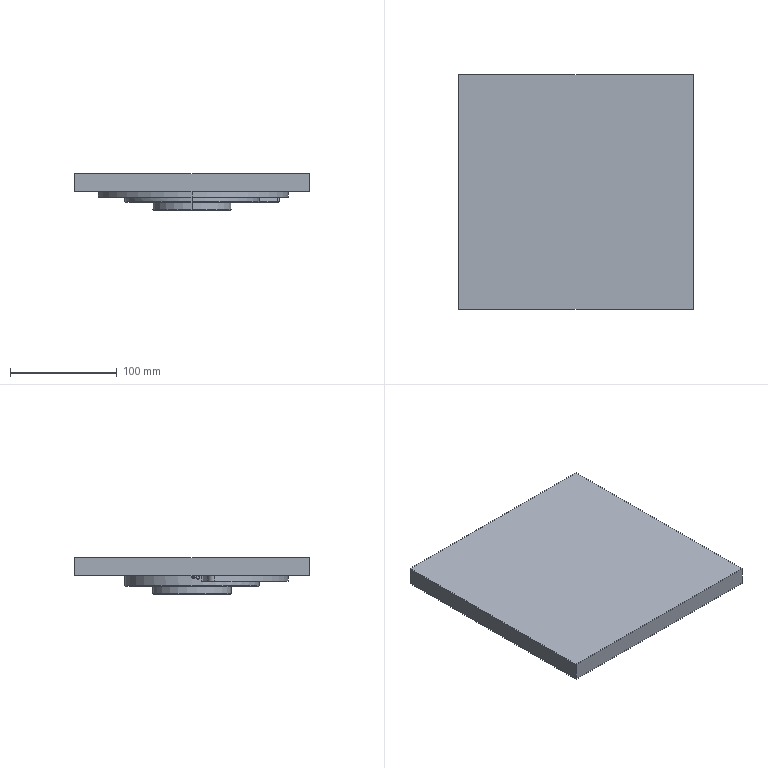NC program | NX | posted with a generic post | part box 220 x 220 x 34.5 mm
Lines 5366 to 5610 of 5610:
(FLOOR_WALL_COPY_COPY , TOOL : D10JING)
N10724 T07 M6
N10726 G54
N10728 G17 G0 G90 X-94.136 Y20.831 S9500 M3
N10730 G43 Z30. H7
N10732 Z-11.
N10734 G94 G1 Z-12.5 F1000.
N10736 X-93.972 Y20.821
N10738 G3 X-92.424 Y21.971 R1.5
N10740 G2 X87.34 Y-37.372 R-95.
N10742 G3 X82.185 Y-28.911 R8.5
N10744 G1 X65. Y-21.616
N10746 G3 X-68.148 Y6.939 R-68.5
N10748 G1 X-84.432 Y9.81
N10750 G2 X-92.424 Y21.971 R10.
N10752 G1 X-86.587 Y20.584
N10754 G2 X85.715 Y-23.956 R-89.
N10756 G3 X84.53 Y-23.388 R14.5
N10758 G1 X72.249 Y-18.175
N10760 G3 X-73.188 Y13.92 R-74.5
N10762 G1 X-83.39 Y15.719
N10764 G2 X-86.587 Y20.584 R4.
N10766 G1 X-80.232 Y21.255
N10768 G2 X81.522 Y-15.593 R83.
N10770 G1 X79.166 Y-14.593
N10772 G3 X-77.761 Y20.819 R80.5
N10774 G1 X-80.232 Y21.255
N10776 G3 X-81.902 Y20.291 R1.5
N10778 G1 Z-11.
N10780 G0 Z30.
N10782 X-69.419 Y3.355
N10784 Z-11.
N10786 G1 Z-12.5
N10788 X-69.173 Y3.38
N10790 G3 X-67.833 Y4.767 R1.5
N10792 G2 X64.379 Y-21.895 R-68.
N10794 G1 X81.99 Y-29.371
N10796 G2 X86.282 Y-39.729 R8.
N10798 G3 X86.879 Y-41.563 R1.5
N10800 G1 X87.042 Y-41.665
N10802 Z-11.
N10804 G0 Z30.
N10806 X-13.604 Y45.122
N10808 Z-16.
N10810 G1 Z-17.5
N10812 G3 X-14.103 Y43.259 R1.5
N10814 G1 X-17.081 Y49.644
N10816 G2 X52.492 Y0.929 R52.5
N10818 G1 X45.474 Y1.543
N10820 G3 X-14.103 Y43.259 R45.5
N10822 G1 X-13.449 Y44.646
N10824 G3 X-13.948 Y42.784 R1.5
N10826 G2 X44.987 Y1.083 R45.
N10828 G1 X52.999 Y0.382
N10830 G3 X-17.767 Y49.933 R53.
N10832 G1 X-14.369 Y42.644
N10834 G2 X-13.948 Y42.784 R45.
N10836 G3 X-12.928 Y44.42 R1.5
N10838 G1 X-12.962 Y44.657
N10840 Z-16.
N10842 G0 Z30.
N10844 M5
(DRILLING_COPY_1_COPY_2 , TOOL : D6A45)
N10846 T18 M6
N10848 G54
N10850 G17 G0 G90 X-28.146 Y-16.25 S3000 M3
N10852 G43 Z30. H18
N10854 G94 G81 G98 Z-1.55 F200. R3.
N10856 X28.146
N10858 X0. Y32.5
N10860 G80
N10862 G0 X0. Y32.5 Z30.
(DRILLING_COPY_1_COPY_2_COPY , TOOL : D6A45)
N10864 X26.5 Y0.
N10866 G81 Z-1.85 F200. R3.
N10868 X13.25 Y22.95
N10870 X-13.25
N10872 X-26.5 Y0.
N10874 X-13.25 Y-22.95
N10876 X13.25
N10878 G80
N10880 G0 X13.25 Y-22.95 Z30.
N10882 M5
(DRILLING_COPY_1_COPY_1_COPY_2 , TOOL : 2.6ZT)
N10884 T12 M6
N10886 G54
N10888 G17 G0 G90 X-28.146 Y-16.25 S3000 M3
N10890 G43 Z30. H12
N10892 G94 G83 G98 Z-8.251 F120. Q2. R3.
N10894 X28.146
N10896 X0. Y32.5
N10898 G80
N10900 G0 X0. Y32.5 Z30.
N10902 M5
(DRILLING_COPY_1_COPY_1_COPY_2_COPY , TOOL : 3.5ZT)
N10904 T17 M6
N10906 G54
N10908 G17 G0 G90 X26.5 Y0. S3000 M3
N10910 G43 Z30. H17
N10912 G94 G83 G98 Z-6.552 F120. Q2. R3.
N10914 X13.25 Y22.95
N10916 X-13.25
N10918 X-26.5 Y0.
N10920 X-13.25 Y-22.95
N10922 X13.25
N10924 G80
N10926 G0 X13.25 Y-22.95 Z30.
N10928 M5
(ZLEVEL_PROFILE_COPY_1_COPY_COPY_COPY_COPY_2_COPY_COPY_COPY , TOOL : D6A45)
N10930 T18 M6
N10932 G54
N10934 G17 G0 G90 X43.577 Y-1.383 S7000 M3
N10936 G43 Z30. H18
N10938 Z-8.5
N10940 G94 G1 X44.143 Y-2.599 F1000.
N10942 G3 X44.635 Y-2.943 R0.6
N10944 G1 X52.646 Y-3.644
N10946 G3 X57.04 Y0.411 R4.041
N10948 X-19.122 Y53.741 R57.041
N10950 X-21.43 Y48.225 R4.041
N10952 G1 X-18.031 Y40.936
N10954 G3 X-13.078 Y38.815 R4.041
N10956 G2 X40.947 Y0.986 R40.959
N10958 G3 X44.635 Y-2.943 R4.041
N10960 X45.179 Y-2.689 R0.6
N10962 G1 X45.775 Y-1.838
N10964 G0 Z30.
N10966 X36.599 Y-37.68
N10968 Z-8.5
N10970 G1 X36.121 Y-38.59
N10972 G3 X36.641 Y-38.89 R0.6
N10974 X37.933 Y-37.599 R1.291
N10976 X36.641 Y-38.89 R-1.291
N10978 X37.161 Y-38.59 R0.6
N10980 G1 X36.684 Y-37.68
N10982 G0 Z30.
N10984 X-34.753 Y40.482
N10986 Z-8.5
N10988 G1 X-35.48 Y41.741
N10990 G3 X-36. Y42.041 R0.6
N10992 G1 X-36.003
N10994 G3 X-39.541 Y38.497 R3.541
N10996 X-36. Y42.041 R-3.541
N10998 X-36.52 Y41.741 R0.6
N11000 G1 X-37.247 Y40.482
N11002 G0 Z30.
N11004 X62.087 Y-24.327
N11006 Z-8.5
N11008 G1 X62.243 Y-25.596
N11010 G3 X62.604 Y-26.076 R0.6
N11012 G1 X80.215 Y-33.551
N11014 G2 X81.999 Y-38.195 R3.459
N11016 X80.864 Y-40.543 R90.459
N11018 X73.255 Y-42.824 R5.459
N11020 G1 X56.036 Y-32.882
N11022 G3 X53.954 Y-33.405 R1.541
N11024 G2 X60.079 Y-20.433 R-63.459
N11026 G3 X62.604 Y-26.076 R4.541
N11028 X63.2 Y-26.003 R0.6
N11030 G1 X64.03 Y-25.377
N11032 G0 Z30.
(ZLEVEL_PROFILE_COPY_1_COPY_COPY_COPY_COPY_2_COPY_COPY_COPY_COPY , TOOL : D6A45)
N11034 X22.903 Y74.945
N11036 Z-13.5
N11038 G1 X23.178 Y75.88
N11040 G3 X22.659 Y76.18 R0.6
N11042 X20.592 Y74.113 R2.066
N11044 X22.659 Y76.18 R-2.066
N11046 X22.139 Y75.88 R0.6
N11048 G1 X22.414 Y74.945
N11050 G0 Z30.
N11052 X57.511 Y52.61
N11054 Z-13.5
N11056 G1 X58.446 Y52.335
N11058 G3 X58.746 Y52.855 R0.6
N11060 X56.68 Y54.921 R2.066
N11062 X58.746 Y52.855 R-2.066
N11064 X58.446 Y53.374 R0.6
N11066 G1 X57.511 Y53.099
N11068 G0 Z30.
N11070 X74.945 Y-22.903
N11072 Z-13.5
N11074 G1 X75.88 Y-23.178
N11076 G3 X76.18 Y-22.659 R0.6
N11078 X74.114 Y-20.592 R2.066
N11080 X76.18 Y-22.659 R-2.066
N11082 X75.88 Y-22.139 R0.6
N11084 G1 X74.945 Y-22.414
N11086 G0 Z30.
N11088 X-34.94 Y69.884
N11090 Z-13.5
N11092 G1 X-34.665 Y70.819
N11094 G3 X-35.184 Y71.119 R0.6
N11096 G1 X-35.192
N11098 G3 X-37.251 Y69.045 R2.066
N11100 X-35.184 Y71.119 R-2.066
N11102 X-35.704 Y70.819 R0.6
N11104 G1 X-35.429 Y69.884
N11106 G0 Z30.
N11108 X76.345 Y17.189
N11110 Z-13.5
N11112 G1 X77.28 Y16.914
N11114 G3 X77.58 Y17.434 R0.6
N11116 X75.514 Y19.5 R2.066
N11118 X77.58 Y17.434 R-2.066
N11120 X77.28 Y17.953 R0.6
N11122 G1 X76.345 Y17.678
N11124 G0 Z30.
N11126 X-72.688 Y29.277
N11128 Z-13.5
N11130 G1 X-73.623 Y29.552
N11132 G3 X-73.923 Y29.032 R0.6
N11134 X-71.857 Y26.966 R2.066
N11136 X-73.923 Y29.032 R-2.066
N11138 X-73.623 Y28.512 R0.6
N11140 G1 X-72.688 Y28.788
N11142 G0 Z30.
N11144 X-66.421 Y9.52
N11146 Z-13.5
N11148 G1 X-65.317 Y10.503
N11150 X-65.355 Y10.542
N11152 X-65.404 Y10.565
N11154 X-65.458 Y10.569
N11156 X-83.73 Y13.791
N11158 G2 X-88.492 Y21.037 R5.959
N11160 X84.443 Y-33.805 R-90.959
N11162 G3 X84.529 Y-34.399 R0.6
N11164 G1 X85.954 Y-36.211
N11166 G0 Z30.
N11168 M5
N11170 M2